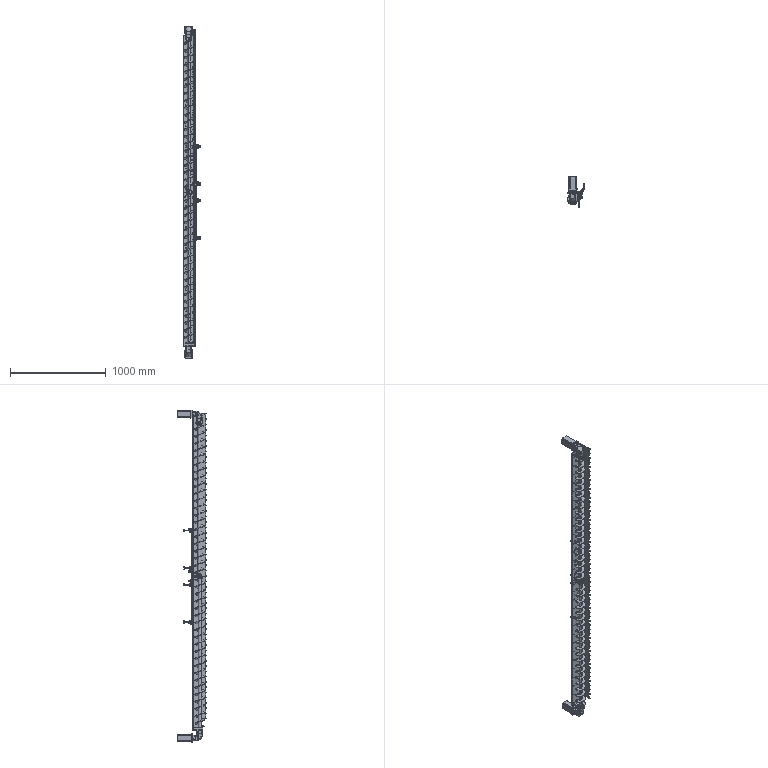Part | 85 solids | 4128 faces | volume 11623934 mm3 | cylinder 1890 | plane 1690 | cone 298 | torus 136 | spline 106 | sphere 8 | commonest cylinder face diameters 4.2 x220 5 x130 4 x124 6 x114 7 x92 6.8 x88